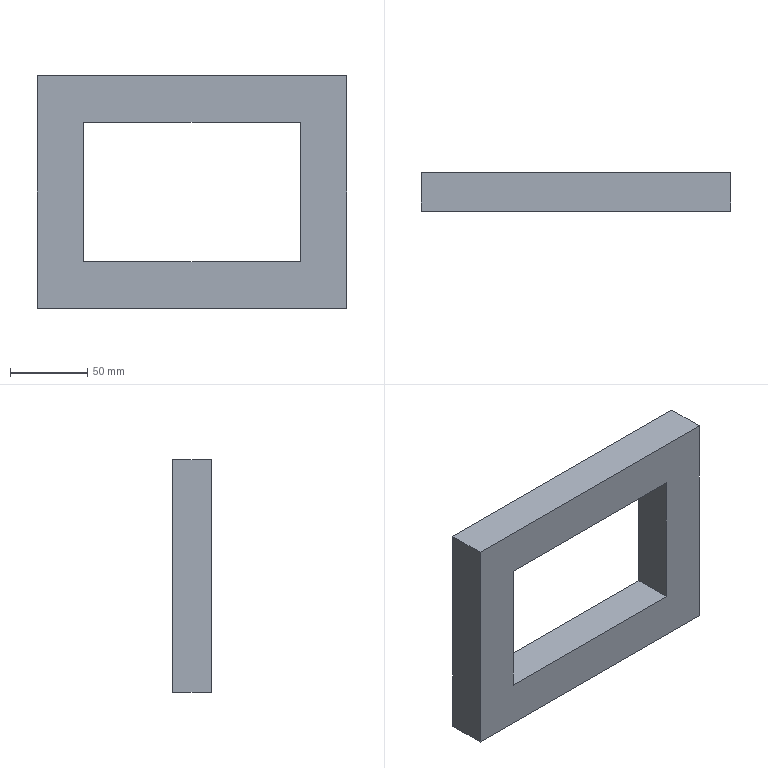Part | SolidWorks | features Extrusion 1, HoleWzd 1, ICE 1 | 1 solid | 46 faces | box 200 x 25 x 150 mm | volume 430967 mm3 | cone 24 | cylinder 12 | plane 10 | commonest cylinder face diameters 6.8 x12
STEP:
#1=CARTESIAN_POINT('',(-85.,24.375,56.6));
#2=VERTEX_POINT('',#1);
#3=CARTESIAN_POINT('',(-85.,24.375,63.4));
#4=VERTEX_POINT('',#3);
#5=CARTESIAN_POINT('',(-85.,24.375,60.));
#6=DIRECTION('',(0.,1.,0.));
#7=DIRECTION('',(0.,0.,1.));
#8=AXIS2_PLACEMENT_3D('',#5,#6,#7);
#9=CIRCLE('',#8,3.4);
#10=EDGE_CURVE('',#2,#4,#9,.T.);
#11=ORIENTED_EDGE('',*,*,#10,.F.);
#12=CARTESIAN_POINT('',(-85.,25.,55.975));
#13=VERTEX_POINT('',#12);
#14=CARTESIAN_POINT('',(-85.,25.,55.975));
#15=DIRECTION('',(0.,0.7071,-0.7071));
#16=VECTOR('',#15,1000.);
#17=LINE('',#14,#16);
#18=EDGE_CURVE('',#2,#13,#17,.T.);
#19=ORIENTED_EDGE('',*,*,#18,.T.);
#20=CARTESIAN_POINT('',(-85.,25.,64.025));
#21=VERTEX_POINT('',#20);
#22=CARTESIAN_POINT('',(-85.,25.,60.));
#23=DIRECTION('',(0.,1.,0.));
#24=DIRECTION('',(0.,0.,1.));
#25=AXIS2_PLACEMENT_3D('',#22,#23,#24);
#26=CIRCLE('',#25,4.025);
#27=EDGE_CURVE('',#13,#21,#26,.T.);
#28=ORIENTED_EDGE('',*,*,#27,.T.);
#29=CARTESIAN_POINT('',(-85.,25.,64.025));
#30=DIRECTION('',(0.,0.7071,0.7071));
#31=VECTOR('',#30,1000.);
#32=LINE('',#29,#31);
#33=EDGE_CURVE('',#4,#21,#32,.T.);
#34=ORIENTED_EDGE('',*,*,#33,.F.);
#35=EDGE_LOOP('',(#11,#19,#28,#34));
#36=FACE_OUTER_BOUND('',#35,.T.);
#37=CARTESIAN_POINT('',(-85.,25.,60.));
#38=DIRECTION('',(0.,1.,0.));
#39=DIRECTION('',(0.,0.,1.));
#40=AXIS2_PLACEMENT_3D('',#37,#38,#39);
#41=CONICAL_SURFACE('',#40,4.025,0.7854);
#42=ADVANCED_FACE('',(#36),#41,.F.);
#43=CARTESIAN_POINT('',(-85.,7.293,56.6));
#44=VERTEX_POINT('',#43);
#45=CARTESIAN_POINT('',(-85.,7.293,63.4));
#46=VERTEX_POINT('',#45);
#47=CARTESIAN_POINT('',(-85.,7.293,60.));
#48=DIRECTION('',(0.,1.,0.));
#49=DIRECTION('',(0.,0.,1.));
#50=AXIS2_PLACEMENT_3D('',#47,#48,#49);
#51=CIRCLE('',#50,3.4);
#52=EDGE_CURVE('',#44,#46,#51,.T.);
#53=ORIENTED_EDGE('',*,*,#52,.F.);
#54=CARTESIAN_POINT('',(-85.,25.,56.6));
#55=DIRECTION('',(0.,1.,0.));
#56=VECTOR('',#55,1000.);
#57=LINE('',#54,#56);
#58=EDGE_CURVE('',#44,#2,#57,.T.);
#59=ORIENTED_EDGE('',*,*,#58,.T.);
#60=ORIENTED_EDGE('',*,*,#10,.T.);
#61=CARTESIAN_POINT('',(-85.,25.,63.4));
#62=DIRECTION('',(0.,1.,0.));
#63=VECTOR('',#62,1000.);
#64=LINE('',#61,#63);
#65=EDGE_CURVE('',#46,#4,#64,.T.);
#66=ORIENTED_EDGE('',*,*,#65,.F.);
#67=EDGE_LOOP('',(#53,#59,#60,#66));
#68=FACE_OUTER_BOUND('',#67,.T.);
#69=CARTESIAN_POINT('',(-85.,25.,60.));
#70=DIRECTION('',(0.,1.,0.));
#71=DIRECTION('',(0.,0.,1.));
#72=AXIS2_PLACEMENT_3D('',#69,#70,#71);
#73=CYLINDRICAL_SURFACE('',#72,3.4);
#74=ADVANCED_FACE('',(#68),#73,.F.);
#75=CARTESIAN_POINT('',(-85.,5.25,60.));
#76=VERTEX_POINT('',#75);
#77=CARTESIAN_POINT('',(-85.,7.293,63.4));
#78=DIRECTION('',(0.,0.515,0.8572));
#79=VECTOR('',#78,1000.);
#80=LINE('',#77,#79);
#81=EDGE_CURVE('',#76,#46,#80,.T.);
#82=ORIENTED_EDGE('',*,*,#81,.F.);
#83=CARTESIAN_POINT('',(-85.,7.293,56.6));
#84=DIRECTION('',(0.,0.515,-0.8572));
#85=VECTOR('',#84,1000.);
#86=LINE('',#83,#85);
#87=EDGE_CURVE('',#76,#44,#86,.T.);
#88=ORIENTED_EDGE('',*,*,#87,.T.);
#89=ORIENTED_EDGE('',*,*,#52,.T.);
#90=EDGE_LOOP('',(#82,#88,#89));
#91=FACE_OUTER_BOUND('',#90,.T.);
#92=CARTESIAN_POINT('',(-85.,7.293,60.));
#93=DIRECTION('',(0.,1.,0.));
#94=DIRECTION('',(0.,0.,1.));
#95=AXIS2_PLACEMENT_3D('',#92,#93,#94);
#96=CONICAL_SURFACE('',#95,3.4,1.03);
#97=ADVANCED_FACE('',(#91),#96,.F.);
#98=CARTESIAN_POINT('',(0.,24.375,56.6));
#99=VERTEX_POINT('',#98);
#100=CARTESIAN_POINT('',(0.,24.375,63.4));
#101=VERTEX_POINT('',#100);
#102=CARTESIAN_POINT('',(0.,24.375,60.));
#103=DIRECTION('',(0.,1.,0.));
#104=DIRECTION('',(0.,0.,1.));
#105=AXIS2_PLACEMENT_3D('',#102,#103,#104);
#106=CIRCLE('',#105,3.4);
#107=EDGE_CURVE('',#99,#101,#106,.T.);
#108=ORIENTED_EDGE('',*,*,#107,.F.);
#109=CARTESIAN_POINT('',(0.,25.,55.975));
#110=VERTEX_POINT('',#109);
#111=CARTESIAN_POINT('',(0.,25.,55.975));
#112=DIRECTION('',(0.,0.7071,-0.7071));
#113=VECTOR('',#112,1000.);
#114=LINE('',#111,#113);
#115=EDGE_CURVE('',#99,#110,#114,.T.);
#116=ORIENTED_EDGE('',*,*,#115,.T.);
#117=CARTESIAN_POINT('',(0.,25.,64.025));
#118=VERTEX_POINT('',#117);
#119=CARTESIAN_POINT('',(0.,25.,60.));
#120=DIRECTION('',(0.,1.,0.));
#121=DIRECTION('',(0.,0.,1.));
#122=AXIS2_PLACEMENT_3D('',#119,#120,#121);
#123=CIRCLE('',#122,4.025);
#124=EDGE_CURVE('',#110,#118,#123,.T.);
#125=ORIENTED_EDGE('',*,*,#124,.T.);
#126=CARTESIAN_POINT('',(0.,25.,64.025));
#127=DIRECTION('',(0.,0.7071,0.7071));
#128=VECTOR('',#127,1000.);
#129=LINE('',#126,#128);
#130=EDGE_CURVE('',#101,#118,#129,.T.);
#131=ORIENTED_EDGE('',*,*,#130,.F.);
#132=EDGE_LOOP('',(#108,#116,#125,#131));
#133=FACE_OUTER_BOUND('',#132,.T.);
#134=CARTESIAN_POINT('',(0.,25.,60.));
#135=DIRECTION('',(0.,1.,0.));
#136=DIRECTION('',(0.,0.,1.));
#137=AXIS2_PLACEMENT_3D('',#134,#135,#136);
#138=CONICAL_SURFACE('',#137,4.025,0.7854);
#139=ADVANCED_FACE('',(#133),#138,.F.);
#140=CARTESIAN_POINT('',(0.,7.293,56.6));
#141=VERTEX_POINT('',#140);
#142=CARTESIAN_POINT('',(0.,7.293,63.4));
#143=VERTEX_POINT('',#142);
#144=CARTESIAN_POINT('',(0.,7.293,60.));
#145=DIRECTION('',(0.,1.,0.));
#146=DIRECTION('',(0.,0.,1.));
#147=AXIS2_PLACEMENT_3D('',#144,#145,#146);
#148=CIRCLE('',#147,3.4);
#149=EDGE_CURVE('',#141,#143,#148,.T.);
#150=ORIENTED_EDGE('',*,*,#149,.F.);
#151=CARTESIAN_POINT('',(0.,25.,56.6));
#152=DIRECTION('',(0.,1.,0.));
#153=VECTOR('',#152,1000.);
#154=LINE('',#151,#153);
#155=EDGE_CURVE('',#141,#99,#154,.T.);
#156=ORIENTED_EDGE('',*,*,#155,.T.);
#157=ORIENTED_EDGE('',*,*,#107,.T.);
#158=CARTESIAN_POINT('',(0.,25.,63.4));
#159=DIRECTION('',(0.,1.,0.));
#160=VECTOR('',#159,1000.);
#161=LINE('',#158,#160);
#162=EDGE_CURVE('',#143,#101,#161,.T.);
#163=ORIENTED_EDGE('',*,*,#162,.F.);
#164=EDGE_LOOP('',(#150,#156,#157,#163));
#165=FACE_OUTER_BOUND('',#164,.T.);
#166=CARTESIAN_POINT('',(0.,25.,60.));
#167=DIRECTION('',(0.,1.,0.));
#168=DIRECTION('',(0.,0.,1.));
#169=AXIS2_PLACEMENT_3D('',#166,#167,#168);
#170=CYLINDRICAL_SURFACE('',#169,3.4);
#171=ADVANCED_FACE('',(#165),#170,.F.);
#172=CARTESIAN_POINT('',(0.,5.25,60.));
#173=VERTEX_POINT('',#172);
#174=CARTESIAN_POINT('',(0.,7.293,63.4));
#175=DIRECTION('',(0.,0.515,0.8572));
#176=VECTOR('',#175,1000.);
#177=LINE('',#174,#176);
#178=EDGE_CURVE('',#173,#143,#177,.T.);
#179=ORIENTED_EDGE('',*,*,#178,.F.);
#180=CARTESIAN_POINT('',(0.,7.293,56.6));
#181=DIRECTION('',(0.,0.515,-0.8572));
#182=VECTOR('',#181,1000.);
#183=LINE('',#180,#182);
#184=EDGE_CURVE('',#173,#141,#183,.T.);
#185=ORIENTED_EDGE('',*,*,#184,.T.);
#186=ORIENTED_EDGE('',*,*,#149,.T.);
#187=EDGE_LOOP('',(#179,#185,#186));
#188=FACE_OUTER_BOUND('',#187,.T.);
#189=CARTESIAN_POINT('',(0.,7.293,60.));
#190=DIRECTION('',(0.,1.,0.));
#191=DIRECTION('',(0.,0.,1.));
#192=AXIS2_PLACEMENT_3D('',#189,#190,#191);
#193=CONICAL_SURFACE('',#192,3.4,1.03);
#194=ADVANCED_FACE('',(#188),#193,.F.);
#195=CARTESIAN_POINT('',(85.,24.375,56.6));
#196=VERTEX_POINT('',#195);
#197=CARTESIAN_POINT('',(85.,24.375,63.4));
#198=VERTEX_POINT('',#197);
#199=CARTESIAN_POINT('',(85.,24.375,60.));
#200=DIRECTION('',(0.,1.,0.));
#201=DIRECTION('',(0.,0.,1.));
#202=AXIS2_PLACEMENT_3D('',#199,#200,#201);
#203=CIRCLE('',#202,3.4);
#204=EDGE_CURVE('',#196,#198,#203,.T.);
#205=ORIENTED_EDGE('',*,*,#204,.F.);
#206=CARTESIAN_POINT('',(85.,25.,55.975));
#207=VERTEX_POINT('',#206);
#208=CARTESIAN_POINT('',(85.,25.,55.975));
#209=DIRECTION('',(0.,0.7071,-0.7071));
#210=VECTOR('',#209,1000.);
#211=LINE('',#208,#210);
#212=EDGE_CURVE('',#196,#207,#211,.T.);
#213=ORIENTED_EDGE('',*,*,#212,.T.);
#214=CARTESIAN_POINT('',(85.,25.,64.025));
#215=VERTEX_POINT('',#214);
#216=CARTESIAN_POINT('',(85.,25.,60.));
#217=DIRECTION('',(0.,1.,0.));
#218=DIRECTION('',(0.,0.,1.));
#219=AXIS2_PLACEMENT_3D('',#216,#217,#218);
#220=CIRCLE('',#219,4.025);
#221=EDGE_CURVE('',#207,#215,#220,.T.);
#222=ORIENTED_EDGE('',*,*,#221,.T.);
#223=CARTESIAN_POINT('',(85.,25.,64.025));
#224=DIRECTION('',(0.,0.7071,0.7071));
#225=VECTOR('',#224,1000.);
#226=LINE('',#223,#225);
#227=EDGE_CURVE('',#198,#215,#226,.T.);
#228=ORIENTED_EDGE('',*,*,#227,.F.);
#229=EDGE_LOOP('',(#205,#213,#222,#228));
#230=FACE_OUTER_BOUND('',#229,.T.);
#231=CARTESIAN_POINT('',(85.,25.,60.));
#232=DIRECTION('',(0.,1.,0.));
#233=DIRECTION('',(0.,0.,1.));
#234=AXIS2_PLACEMENT_3D('',#231,#232,#233);
#235=CONICAL_SURFACE('',#234,4.025,0.7854);
#236=ADVANCED_FACE('',(#230),#235,.F.);
#237=CARTESIAN_POINT('',(85.,7.293,56.6));
#238=VERTEX_POINT('',#237);
#239=CARTESIAN_POINT('',(85.,7.293,63.4));
#240=VERTEX_POINT('',#239);
#241=CARTESIAN_POINT('',(85.,7.293,60.));
#242=DIRECTION('',(0.,1.,0.));
#243=DIRECTION('',(0.,0.,1.));
#244=AXIS2_PLACEMENT_3D('',#241,#242,#243);
#245=CIRCLE('',#244,3.4);
#246=EDGE_CURVE('',#238,#240,#245,.T.);
#247=ORIENTED_EDGE('',*,*,#246,.F.);
#248=CARTESIAN_POINT('',(85.,25.,56.6));
#249=DIRECTION('',(0.,1.,0.));
#250=VECTOR('',#249,1000.);
#251=LINE('',#248,#250);
#252=EDGE_CURVE('',#238,#196,#251,.T.);
#253=ORIENTED_EDGE('',*,*,#252,.T.);
#254=ORIENTED_EDGE('',*,*,#204,.T.);
#255=CARTESIAN_POINT('',(85.,25.,63.4));
#256=DIRECTION('',(0.,1.,0.));
#257=VECTOR('',#256,1000.);
#258=LINE('',#255,#257);
#259=EDGE_CURVE('',#240,#198,#258,.T.);
#260=ORIENTED_EDGE('',*,*,#259,.F.);
#261=EDGE_LOOP('',(#247,#253,#254,#260));
#262=FACE_OUTER_BOUND('',#261,.T.);
#263=CARTESIAN_POINT('',(85.,25.,60.));
#264=DIRECTION('',(0.,1.,0.));
#265=DIRECTION('',(0.,0.,1.));
#266=AXIS2_PLACEMENT_3D('',#263,#264,#265);
#267=CYLINDRICAL_SURFACE('',#266,3.4);
#268=ADVANCED_FACE('',(#262),#267,.F.);
#269=CARTESIAN_POINT('',(85.,5.25,60.));
#270=VERTEX_POINT('',#269);
#271=CARTESIAN_POINT('',(85.,7.293,63.4));
#272=DIRECTION('',(0.,0.515,0.8572));
#273=VECTOR('',#272,1000.);
#274=LINE('',#271,#273);
#275=EDGE_CURVE('',#270,#240,#274,.T.);
#276=ORIENTED_EDGE('',*,*,#275,.F.);
#277=CARTESIAN_POINT('',(85.,7.293,56.6));
#278=DIRECTION('',(0.,0.515,-0.8572));
#279=VECTOR('',#278,1000.);
#280=LINE('',#277,#279);
#281=EDGE_CURVE('',#270,#238,#280,.T.);
#282=ORIENTED_EDGE('',*,*,#281,.T.);
#283=ORIENTED_EDGE('',*,*,#246,.T.);
#284=EDGE_LOOP('',(#276,#282,#283));
#285=FACE_OUTER_BOUND('',#284,.T.);
#286=CARTESIAN_POINT('',(85.,7.293,60.));
#287=DIRECTION('',(0.,1.,0.));
#288=DIRECTION('',(0.,0.,1.));
#289=AXIS2_PLACEMENT_3D('',#286,#287,#288);
#290=CONICAL_SURFACE('',#289,3.4,1.03);
#291=ADVANCED_FACE('',(#285),#290,.F.);
#292=CARTESIAN_POINT('',(85.,24.375,-63.4));
#293=VERTEX_POINT('',#292);
#294=CARTESIAN_POINT('',(85.,24.375,-56.6));
#295=VERTEX_POINT('',#294);
#296=CARTESIAN_POINT('',(85.,24.375,-60.));
#297=DIRECTION('',(0.,1.,0.));
#298=DIRECTION('',(0.,0.,1.));
#299=AXIS2_PLACEMENT_3D('',#296,#297,#298);
#300=CIRCLE('',#299,3.4);
#301=EDGE_CURVE('',#293,#295,#300,.T.);
#302=ORIENTED_EDGE('',*,*,#301,.F.);
#303=CARTESIAN_POINT('',(85.,25.,-64.025));
#304=VERTEX_POINT('',#303);
#305=CARTESIAN_POINT('',(85.,25.,-64.025));
#306=DIRECTION('',(0.,0.7071,-0.7071));
#307=VECTOR('',#306,1000.);
#308=LINE('',#305,#307);
#309=EDGE_CURVE('',#293,#304,#308,.T.);
#310=ORIENTED_EDGE('',*,*,#309,.T.);
#311=CARTESIAN_POINT('',(85.,25.,-55.975));
#312=VERTEX_POINT('',#311);
#313=CARTESIAN_POINT('',(85.,25.,-60.));
#314=DIRECTION('',(0.,1.,0.));
#315=DIRECTION('',(0.,0.,1.));
#316=AXIS2_PLACEMENT_3D('',#313,#314,#315);
#317=CIRCLE('',#316,4.025);
#318=EDGE_CURVE('',#304,#312,#317,.T.);
#319=ORIENTED_EDGE('',*,*,#318,.T.);
#320=CARTESIAN_POINT('',(85.,25.,-55.975));
#321=DIRECTION('',(0.,0.7071,0.7071));
#322=VECTOR('',#321,1000.);
#323=LINE('',#320,#322);
#324=EDGE_CURVE('',#295,#312,#323,.T.);
#325=ORIENTED_EDGE('',*,*,#324,.F.);
#326=EDGE_LOOP('',(#302,#310,#319,#325));
#327=FACE_OUTER_BOUND('',#326,.T.);
#328=CARTESIAN_POINT('',(85.,25.,-60.));
#329=DIRECTION('',(0.,1.,0.));
#330=DIRECTION('',(0.,0.,1.));
#331=AXIS2_PLACEMENT_3D('',#328,#329,#330);
#332=CONICAL_SURFACE('',#331,4.025,0.7854);
#333=ADVANCED_FACE('',(#327),#332,.F.);
#334=CARTESIAN_POINT('',(85.,7.293,-63.4));
#335=VERTEX_POINT('',#334);
#336=CARTESIAN_POINT('',(85.,7.293,-56.6));
#337=VERTEX_POINT('',#336);
#338=CARTESIAN_POINT('',(85.,7.293,-60.));
#339=DIRECTION('',(0.,1.,0.));
#340=DIRECTION('',(0.,0.,1.));
#341=AXIS2_PLACEMENT_3D('',#338,#339,#340);
#342=CIRCLE('',#341,3.4);
#343=EDGE_CURVE('',#335,#337,#342,.T.);
#344=ORIENTED_EDGE('',*,*,#343,.F.);
#345=CARTESIAN_POINT('',(85.,25.,-63.4));
#346=DIRECTION('',(0.,1.,0.));
#347=VECTOR('',#346,1000.);
#348=LINE('',#345,#347);
#349=EDGE_CURVE('',#335,#293,#348,.T.);
#350=ORIENTED_EDGE('',*,*,#349,.T.);
#351=ORIENTED_EDGE('',*,*,#301,.T.);
#352=CARTESIAN_POINT('',(85.,25.,-56.6));
#353=DIRECTION('',(0.,1.,0.));
#354=VECTOR('',#353,1000.);
#355=LINE('',#352,#354);
#356=EDGE_CURVE('',#337,#295,#355,.T.);
#357=ORIENTED_EDGE('',*,*,#356,.F.);
#358=EDGE_LOOP('',(#344,#350,#351,#357));
#359=FACE_OUTER_BOUND('',#358,.T.);
#360=CARTESIAN_POINT('',(85.,25.,-60.));
#361=DIRECTION('',(0.,1.,0.));
#362=DIRECTION('',(0.,0.,1.));
#363=AXIS2_PLACEMENT_3D('',#360,#361,#362);
#364=CYLINDRICAL_SURFACE('',#363,3.4);
#365=ADVANCED_FACE('',(#359),#364,.F.);
#366=CARTESIAN_POINT('',(85.,5.25,-60.));
#367=VERTEX_POINT('',#366);
#368=CARTESIAN_POINT('',(85.,7.293,-56.6));
#369=DIRECTION('',(0.,0.515,0.8572));
#370=VECTOR('',#369,1000.);
#371=LINE('',#368,#370);
#372=EDGE_CURVE('',#367,#337,#371,.T.);
#373=ORIENTED_EDGE('',*,*,#372,.F.);
#374=CARTESIAN_POINT('',(85.,7.293,-63.4));
#375=DIRECTION('',(0.,0.515,-0.8572));
#376=VECTOR('',#375,1000.);
#377=LINE('',#374,#376);
#378=EDGE_CURVE('',#367,#335,#377,.T.);
#379=ORIENTED_EDGE('',*,*,#378,.T.);
#380=ORIENTED_EDGE('',*,*,#343,.T.);
#381=EDGE_LOOP('',(#373,#379,#380));
#382=FACE_OUTER_BOUND('',#381,.T.);
#383=CARTESIAN_POINT('',(85.,7.293,-60.));
#384=DIRECTION('',(0.,1.,0.));
#385=DIRECTION('',(0.,0.,1.));
#386=AXIS2_PLACEMENT_3D('',#383,#384,#385);
#387=CONICAL_SURFACE('',#386,3.4,1.03);
#388=ADVANCED_FACE('',(#382),#387,.F.);
#389=CARTESIAN_POINT('',(0.,24.375,-63.4));
#390=VERTEX_POINT('',#389);
#391=CARTESIAN_POINT('',(0.,24.375,-56.6));
#392=VERTEX_POINT('',#391);
#393=CARTESIAN_POINT('',(0.,24.375,-60.));
#394=DIRECTION('',(0.,1.,0.));
#395=DIRECTION('',(0.,0.,1.));
#396=AXIS2_PLACEMENT_3D('',#393,#394,#395);
#397=CIRCLE('',#396,3.4);
#398=EDGE_CURVE('',#390,#392,#397,.T.);
#399=ORIENTED_EDGE('',*,*,#398,.F.);
#400=CARTESIAN_POINT('',(0.,25.,-64.025));
#401=VERTEX_POINT('',#400);
#402=CARTESIAN_POINT('',(0.,25.,-64.025));
#403=DIRECTION('',(0.,0.7071,-0.7071));
#404=VECTOR('',#403,1000.);
#405=LINE('',#402,#404);
#406=EDGE_CURVE('',#390,#401,#405,.T.);
#407=ORIENTED_EDGE('',*,*,#406,.T.);
#408=CARTESIAN_POINT('',(0.,25.,-55.975));
#409=VERTEX_POINT('',#408);
#410=CARTESIAN_POINT('',(0.,25.,-60.));
#411=DIRECTION('',(0.,1.,0.));
#412=DIRECTION('',(0.,0.,1.));
#413=AXIS2_PLACEMENT_3D('',#410,#411,#412);
#414=CIRCLE('',#413,4.025);
#415=EDGE_CURVE('',#401,#409,#414,.T.);
#416=ORIENTED_EDGE('',*,*,#415,.T.);
#417=CARTESIAN_POINT('',(0.,25.,-55.975));
#418=DIRECTION('',(0.,0.7071,0.7071));
#419=VECTOR('',#418,1000.);
#420=LINE('',#417,#419);
#421=EDGE_CURVE('',#392,#409,#420,.T.);
#422=ORIENTED_EDGE('',*,*,#421,.F.);
#423=EDGE_LOOP('',(#399,#407,#416,#422));
#424=FACE_OUTER_BOUND('',#423,.T.);
#425=CARTESIAN_POINT('',(0.,25.,-60.));
#426=DIRECTION('',(0.,1.,0.));
#427=DIRECTION('',(0.,0.,1.));
#428=AXIS2_PLACEMENT_3D('',#425,#426,#427);
#429=CONICAL_SURFACE('',#428,4.025,0.7854);
#430=ADVANCED_FACE('',(#424),#429,.F.);
#431=CARTESIAN_POINT('',(0.,7.293,-63.4));
#432=VERTEX_POINT('',#431);
#433=CARTESIAN_POINT('',(0.,7.293,-56.6));
#434=VERTEX_POINT('',#433);
#435=CARTESIAN_POINT('',(0.,7.293,-60.));
#436=DIRECTION('',(0.,1.,0.));
#437=DIRECTION('',(0.,0.,1.));
#438=AXIS2_PLACEMENT_3D('',#435,#436,#437);
#439=CIRCLE('',#438,3.4);
#440=EDGE_CURVE('',#432,#434,#439,.T.);
#441=ORIENTED_EDGE('',*,*,#440,.F.);
#442=CARTESIAN_POINT('',(0.,25.,-63.4));
#443=DIRECTION('',(0.,1.,0.));
#444=VECTOR('',#443,1000.);
#445=LINE('',#442,#444);
#446=EDGE_CURVE('',#432,#390,#445,.T.);
#447=ORIENTED_EDGE('',*,*,#446,.T.);
#448=ORIENTED_EDGE('',*,*,#398,.T.);
#449=CARTESIAN_POINT('',(0.,25.,-56.6));
#450=DIRECTION('',(0.,1.,0.));
#451=VECTOR('',#450,1000.);
#452=LINE('',#449,#451);
#453=EDGE_CURVE('',#434,#392,#452,.T.);
#454=ORIENTED_EDGE('',*,*,#453,.F.);
#455=EDGE_LOOP('',(#441,#447,#448,#454));
#456=FACE_OUTER_BOUND('',#455,.T.);
#457=CARTESIAN_POINT('',(0.,25.,-60.));
#458=DIRECTION('',(0.,1.,0.));
#459=DIRECTION('',(0.,0.,1.));
#460=AXIS2_PLACEMENT_3D('',#457,#458,#459);
#461=CYLINDRICAL_SURFACE('',#460,3.4);
#462=ADVANCED_FACE('',(#456),#461,.F.);
#463=CARTESIAN_POINT('',(0.,5.25,-60.));
#464=VERTEX_POINT('',#463);
#465=CARTESIAN_POINT('',(0.,7.293,-56.6));
#466=DIRECTION('',(0.,0.515,0.8572));
#467=VECTOR('',#466,1000.);
#468=LINE('',#465,#467);
#469=EDGE_CURVE('',#464,#434,#468,.T.);
#470=ORIENTED_EDGE('',*,*,#469,.F.);
#471=CARTESIAN_POINT('',(0.,7.293,-63.4));
#472=DIRECTION('',(0.,0.515,-0.8572));
#473=VECTOR('',#472,1000.);
#474=LINE('',#471,#473);
#475=EDGE_CURVE('',#464,#432,#474,.T.);
#476=ORIENTED_EDGE('',*,*,#475,.T.);
#477=ORIENTED_EDGE('',*,*,#440,.T.);
#478=EDGE_LOOP('',(#470,#476,#477));
#479=FACE_OUTER_BOUND('',#478,.T.);
#480=CARTESIAN_POINT('',(0.,7.293,-60.));
#481=DIRECTION('',(0.,1.,0.));
#482=DIRECTION('',(0.,0.,1.));
#483=AXIS2_PLACEMENT_3D('',#480,#481,#482);
#484=CONICAL_SURFACE('',#483,3.4,1.03);
#485=ADVANCED_FACE('',(#479),#484,.F.);
#486=CARTESIAN_POINT('',(-85.,24.375,-63.4));
#487=VERTEX_POINT('',#486);
#488=CARTESIAN_POINT('',(-85.,24.375,-56.6));
#489=VERTEX_POINT('',#488);
#490=CARTESIAN_POINT('',(-85.,24.375,-60.));
#491=DIRECTION('',(0.,1.,0.));
#492=DIRECTION('',(0.,0.,1.));
#493=AXIS2_PLACEMENT_3D('',#490,#491,#492);
#494=CIRCLE('',#493,3.4);
#495=EDGE_CURVE('',#487,#489,#494,.T.);
#496=ORIENTED_EDGE('',*,*,#495,.F.);
#497=CARTESIAN_POINT('',(-85.,25.,-64.025));
#498=VERTEX_POINT('',#497);
#499=CARTESIAN_POINT('',(-85.,25.,-64.025));
#500=DIRECTION('',(0.,0.7071,-0.7071));
#501=VECTOR('',#500,1000.);
#502=LINE('',#499,#501);
#503=EDGE_CURVE('',#487,#498,#502,.T.);
#504=ORIENTED_EDGE('',*,*,#503,.T.);
#505=CARTESIAN_POINT('',(-85.,25.,-55.975));
#506=VERTEX_POINT('',#505);
#507=CARTESIAN_POINT('',(-85.,25.,-60.));
#508=DIRECTION('',(0.,1.,0.));
#509=DIRECTION('',(0.,0.,1.));
#510=AXIS2_PLACEMENT_3D('',#507,#508,#509);
#511=CIRCLE('',#510,4.025);
#512=EDGE_CURVE('',#498,#506,#511,.T.);
#513=ORIENTED_EDGE('',*,*,#512,.T.);
#514=CARTESIAN_POINT('',(-85.,25.,-55.975));
#515=DIRECTION('',(0.,0.7071,0.7071));
#516=VECTOR('',#515,1000.);
#517=LINE('',#514,#516);
#518=EDGE_CURVE('',#489,#506,#517,.T.);
#519=ORIENTED_EDGE('',*,*,#518,.F.);
#520=EDGE_LOOP('',(#496,#504,#513,#519));
#521=FACE_OUTER_BOUND('',#520,.T.);
#522=CARTESIAN_POINT('',(-85.,25.,-60.));
#523=DIRECTION('',(0.,1.,0.));
#524=DIRECTION('',(0.,0.,1.));
#525=AXIS2_PLACEMENT_3D('',#522,#523,#524);
#526=CONICAL_SURFACE('',#525,4.025,0.7854);
#527=ADVANCED_FACE('',(#521),#526,.F.);
#528=CARTESIAN_POINT('',(-85.,7.293,-63.4));
#529=VERTEX_POINT('',#528);
#530=CARTESIAN_POINT('',(-85.,7.293,-56.6));
#531=VERTEX_POINT('',#530);
#532=CARTESIAN_POINT('',(-85.,7.293,-60.));
#533=DIRECTION('',(0.,1.,0.));
#534=DIRECTION('',(0.,0.,1.));
#535=AXIS2_PLACEMENT_3D('',#532,#533,#534);
#536=CIRCLE('',#535,3.4);
#537=EDGE_CURVE('',#529,#531,#536,.T.);
#538=ORIENTED_EDGE('',*,*,#537,.F.);
#539=CARTESIAN_POINT('',(-85.,25.,-63.4));
#540=DIRECTION('',(0.,1.,0.));
#541=VECTOR('',#540,1000.);
#542=LINE('',#539,#541);
#543=EDGE_CURVE('',#529,#487,#542,.T.);
#544=ORIENTED_EDGE('',*,*,#543,.T.);
#545=ORIENTED_EDGE('',*,*,#495,.T.);
#546=CARTESIAN_POINT('',(-85.,25.,-56.6));
#547=DIRECTION('',(0.,1.,0.));
#548=VECTOR('',#547,1000.);
#549=LINE('',#546,#548);
#550=EDGE_CURVE('',#531,#489,#549,.T.);
#551=ORIENTED_EDGE('',*,*,#550,.F.);
#552=EDGE_LOOP('',(#538,#544,#545,#551));
#553=FACE_OUTER_BOUND('',#552,.T.);
#554=CARTESIAN_POINT('',(-85.,25.,-60.));
#555=DIRECTION('',(0.,1.,0.));
#556=DIRECTION('',(0.,0.,1.));
#557=AXIS2_PLACEMENT_3D('',#554,#555,#556);
#558=CYLINDRICAL_SURFACE('',#557,3.4);
#559=ADVANCED_FACE('',(#553),#558,.F.);
#560=CARTESIAN_POINT('',(-85.,5.25,-60.));
#561=VERTEX_POINT('',#560);
#562=CARTESIAN_POINT('',(-85.,7.293,-56.6));
#563=DIRECTION('',(0.,0.515,0.8572));
#564=VECTOR('',#563,1000.);
#565=LINE('',#562,#564);
#566=EDGE_CURVE('',#561,#531,#565,.T.);
#567=ORIENTED_EDGE('',*,*,#566,.F.);
#568=CARTESIAN_POINT('',(-85.,7.293,-63.4));
#569=DIRECTION('',(0.,0.515,-0.8572));
#570=VECTOR('',#569,1000.);
#571=LINE('',#568,#570);
#572=EDGE_CURVE('',#561,#529,#571,.T.);
#573=ORIENTED_EDGE('',*,*,#572,.T.);
#574=ORIENTED_EDGE('',*,*,#537,.T.);
#575=EDGE_LOOP('',(#567,#573,#574));
#576=FACE_OUTER_BOUND('',#575,.T.);
#577=CARTESIAN_POINT('',(-85.,7.293,-60.));
#578=DIRECTION('',(0.,1.,0.));
#579=DIRECTION('',(0.,0.,1.));
#580=AXIS2_PLACEMENT_3D('',#577,#578,#579);
#581=CONICAL_SURFACE('',#580,3.4,1.03);
#582=ADVANCED_FACE('',(#576),#581,.F.);
#583=CARTESIAN_POINT('',(100.,0.,75.));
#584=VERTEX_POINT('',#583);
#585=CARTESIAN_POINT('',(100.,0.,-75.));
#586=VERTEX_POINT('',#585);
#587=CARTESIAN_POINT('',(100.,0.,-75.));
#588=DIRECTION('',(0.,0.,-1.));
#589=VECTOR('',#588,1000.);
#590=LINE('',#587,#589);
#591=EDGE_CURVE('',#584,#586,#590,.T.);
#592=ORIENTED_EDGE('',*,*,#591,.T.);
#593=CARTESIAN_POINT('',(100.,25.,-75.));
#594=VERTEX_POINT('',#593);
#595=CARTESIAN_POINT('',(100.,25.,-75.));
#596=DIRECTION('',(0.,-1.,0.));
#597=VECTOR('',#596,1000.);
#598=LINE('',#595,#597);
#599=EDGE_CURVE('',#594,#586,#598,.T.);
#600=ORIENTED_EDGE('',*,*,#599,.F.);
#601=CARTESIAN_POINT('',(100.,25.,75.));
#602=VERTEX_POINT('',#601);
#603=CARTESIAN_POINT('',(100.,25.,-75.));
#604=DIRECTION('',(0.,0.,-1.));
#605=VECTOR('',#604,1000.);
#606=LINE('',#603,#605);
#607=EDGE_CURVE('',#602,#594,#606,.T.);
#608=ORIENTED_EDGE('',*,*,#607,.F.);
#609=CARTESIAN_POINT('',(100.,25.,75.));
#610=DIRECTION('',(0.,-1.,0.));
#611=VECTOR('',#610,1000.);
#612=LINE('',#609,#611);
#613=EDGE_CURVE('',#602,#584,#612,.T.);
#614=ORIENTED_EDGE('',*,*,#613,.T.);
#615=EDGE_LOOP('',(#592,#600,#608,#614));
#616=FACE_OUTER_BOUND('',#615,.T.);
#617=CARTESIAN_POINT('',(100.,25.,-75.));
#618=DIRECTION('',(-1.,0.,0.));
#619=DIRECTION('',(0.,0.,1.));
#620=AXIS2_PLACEMENT_3D('',#617,#618,#619);
#621=PLANE('',#620);
#622=ADVANCED_FACE('',(#616),#621,.F.);
#623=CARTESIAN_POINT('',(-100.,0.,-75.));
#624=VERTEX_POINT('',#623);
#625=CARTESIAN_POINT('',(-100.,0.,-75.));
#626=DIRECTION('',(-1.,0.,0.));
#627=VECTOR('',#626,1000.);
#628=LINE('',#625,#627);
#629=EDGE_CURVE('',#586,#624,#628,.T.);
#630=ORIENTED_EDGE('',*,*,#629,.T.);
#631=CARTESIAN_POINT('',(-100.,25.,-75.));
#632=VERTEX_POINT('',#631);
#633=CARTESIAN_POINT('',(-100.,25.,-75.));
#634=DIRECTION('',(0.,-1.,0.));
#635=VECTOR('',#634,1000.);
#636=LINE('',#633,#635);
#637=EDGE_CURVE('',#632,#624,#636,.T.);
#638=ORIENTED_EDGE('',*,*,#637,.F.);
#639=CARTESIAN_POINT('',(-100.,25.,-75.));
#640=DIRECTION('',(-1.,0.,0.));
#641=VECTOR('',#640,1000.);
#642=LINE('',#639,#641);
#643=EDGE_CURVE('',#594,#632,#642,.T.);
#644=ORIENTED_EDGE('',*,*,#643,.F.);
#645=ORIENTED_EDGE('',*,*,#599,.T.);
#646=EDGE_LOOP('',(#630,#638,#644,#645));
#647=FACE_OUTER_BOUND('',#646,.T.);
#648=CARTESIAN_POINT('',(-100.,25.,-75.));
#649=DIRECTION('',(0.,0.,1.));
#650=DIRECTION('',(1.,0.,0.));
#651=AXIS2_PLACEMENT_3D('',#648,#649,#650);
#652=PLANE('',#651);
#653=ADVANCED_FACE('',(#647),#652,.F.);
#654=CARTESIAN_POINT('',(-100.,0.,75.));
#655=VERTEX_POINT('',#654);
#656=CARTESIAN_POINT('',(-100.,0.,-75.));
#657=DIRECTION('',(0.,0.,1.));
#658=VECTOR('',#657,1000.);
#659=LINE('',#656,#658);
#660=EDGE_CURVE('',#624,#655,#659,.T.);
#661=ORIENTED_EDGE('',*,*,#660,.T.);
#662=CARTESIAN_POINT('',(-100.,25.,75.));
#663=VERTEX_POINT('',#662);
#664=CARTESIAN_POINT('',(-100.,25.,75.));
#665=DIRECTION('',(0.,-1.,0.));
#666=VECTOR('',#665,1000.);
#667=LINE('',#664,#666);
#668=EDGE_CURVE('',#663,#655,#667,.T.);
#669=ORIENTED_EDGE('',*,*,#668,.F.);
#670=CARTESIAN_POINT('',(-100.,25.,-75.));
#671=DIRECTION('',(0.,0.,1.));
#672=VECTOR('',#671,1000.);
#673=LINE('',#670,#672);
#674=EDGE_CURVE('',#632,#663,#673,.T.);
#675=ORIENTED_EDGE('',*,*,#674,.F.);
#676=ORIENTED_EDGE('',*,*,#637,.T.);
#677=EDGE_LOOP('',(#661,#669,#675,#676));
#678=FACE_OUTER_BOUND('',#677,.T.);
#679=CARTESIAN_POINT('',(-100.,25.,-75.));
#680=DIRECTION('',(1.,0.,0.));
#681=DIRECTION('',(0.,0.,-1.));
#682=AXIS2_PLACEMENT_3D('',#679,#680,#681);
#683=PLANE('',#682);
#684=ADVANCED_FACE('',(#678),#683,.F.);
#685=CARTESIAN_POINT('',(-100.,0.,75.));
#686=DIRECTION('',(1.,0.,0.));
#687=VECTOR('',#686,1000.);
#688=LINE('',#685,#687);
#689=EDGE_CURVE('',#655,#584,#688,.T.);
#690=ORIENTED_EDGE('',*,*,#689,.T.);
#691=ORIENTED_EDGE('',*,*,#613,.F.);
#692=CARTESIAN_POINT('',(-100.,25.,75.));
#693=DIRECTION('',(1.,0.,0.));
#694=VECTOR('',#693,1000.);
#695=LINE('',#692,#694);
#696=EDGE_CURVE('',#663,#602,#695,.T.);
#697=ORIENTED_EDGE('',*,*,#696,.F.);
#698=ORIENTED_EDGE('',*,*,#668,.T.);
#699=EDGE_LOOP('',(#690,#691,#697,#698));
#700=FACE_OUTER_BOUND('',#699,.T.);
#701=CARTESIAN_POINT('',(-100.,25.,75.));
#702=DIRECTION('',(0.,0.,-1.));
#703=DIRECTION('',(-1.,0.,0.));
#704=AXIS2_PLACEMENT_3D('',#701,#702,#703);
#705=PLANE('',#704);
#706=ADVANCED_FACE('',(#700),#705,.F.);
#707=CARTESIAN_POINT('',(-70.,25.,-45.));
#708=VERTEX_POINT('',#707);
#709=CARTESIAN_POINT('',(-70.,25.,45.));
#710=VERTEX_POINT('',#709);
#711=CARTESIAN_POINT('',(-70.,25.,0.));
#712=DIRECTION('',(0.,0.,1.));
#713=VECTOR('',#712,1000.);
#714=LINE('',#711,#713);
#715=EDGE_CURVE('',#708,#710,#714,.T.);
#716=ORIENTED_EDGE('',*,*,#715,.F.);
#717=CARTESIAN_POINT('',(70.,25.,-45.));
#718=VERTEX_POINT('',#717);
#719=CARTESIAN_POINT('',(0.,25.,-45.));
#720=DIRECTION('',(-1.,0.,0.));
#721=VECTOR('',#720,1000.);
#722=LINE('',#719,#721);
#723=EDGE_CURVE('',#718,#708,#722,.T.);
#724=ORIENTED_EDGE('',*,*,#723,.F.);
#725=CARTESIAN_POINT('',(70.,25.,45.));
#726=VERTEX_POINT('',#725);
#727=CARTESIAN_POINT('',(70.,25.,0.));
#728=DIRECTION('',(0.,0.,-1.));
#729=VECTOR('',#728,1000.);
#730=LINE('',#727,#729);
#731=EDGE_CURVE('',#726,#718,#730,.T.);
#732=ORIENTED_EDGE('',*,*,#731,.F.);
#733=CARTESIAN_POINT('',(0.,25.,45.));
#734=DIRECTION('',(1.,0.,0.));
#735=VECTOR('',#734,1000.);
#736=LINE('',#733,#735);
#737=EDGE_CURVE('',#710,#726,#736,.T.);
#738=ORIENTED_EDGE('',*,*,#737,.F.);
#739=EDGE_LOOP('',(#716,#724,#732,#738));
#740=FACE_BOUND('',#739,.T.);
#741=CARTESIAN_POINT('',(-85.,25.,60.));
#742=DIRECTION('',(0.,1.,0.));
#743=DIRECTION('',(0.,0.,1.));
#744=AXIS2_PLACEMENT_3D('',#741,#742,#743);
#745=CIRCLE('',#744,4.025);
#746=EDGE_CURVE('',#21,#13,#745,.T.);
#747=ORIENTED_EDGE('',*,*,#746,.F.);
#748=ORIENTED_EDGE('',*,*,#27,.F.);
#749=EDGE_LOOP('',(#747,#748));
#750=FACE_BOUND('',#749,.T.);
#751=CARTESIAN_POINT('',(0.,25.,60.));
#752=DIRECTION('',(0.,1.,0.));
#753=DIRECTION('',(0.,0.,1.));
#754=AXIS2_PLACEMENT_3D('',#751,#752,#753);
#755=CIRCLE('',#754,4.025);
#756=EDGE_CURVE('',#118,#110,#755,.T.);
#757=ORIENTED_EDGE('',*,*,#756,.F.);
#758=ORIENTED_EDGE('',*,*,#124,.F.);
#759=EDGE_LOOP('',(#757,#758));
#760=FACE_BOUND('',#759,.T.);
#761=CARTESIAN_POINT('',(85.,25.,60.));
#762=DIRECTION('',(0.,1.,0.));
#763=DIRECTION('',(0.,0.,1.));
#764=AXIS2_PLACEMENT_3D('',#761,#762,#763);
#765=CIRCLE('',#764,4.025);
#766=EDGE_CURVE('',#215,#207,#765,.T.);
#767=ORIENTED_EDGE('',*,*,#766,.F.);
#768=ORIENTED_EDGE('',*,*,#221,.F.);
#769=EDGE_LOOP('',(#767,#768));
#770=FACE_BOUND('',#769,.T.);
#771=CARTESIAN_POINT('',(85.,25.,-60.));
#772=DIRECTION('',(0.,1.,0.));
#773=DIRECTION('',(0.,0.,1.));
#774=AXIS2_PLACEMENT_3D('',#771,#772,#773);
#775=CIRCLE('',#774,4.025);
#776=EDGE_CURVE('',#312,#304,#775,.T.);
#777=ORIENTED_EDGE('',*,*,#776,.F.);
#778=ORIENTED_EDGE('',*,*,#318,.F.);
#779=EDGE_LOOP('',(#777,#778));
#780=FACE_BOUND('',#779,.T.);
#781=CARTESIAN_POINT('',(0.,25.,-60.));
#782=DIRECTION('',(0.,1.,0.));
#783=DIRECTION('',(0.,0.,1.));
#784=AXIS2_PLACEMENT_3D('',#781,#782,#783);
#785=CIRCLE('',#784,4.025);
#786=EDGE_CURVE('',#409,#401,#785,.T.);
#787=ORIENTED_EDGE('',*,*,#786,.F.);
#788=ORIENTED_EDGE('',*,*,#415,.F.);
#789=EDGE_LOOP('',(#787,#788));
#790=FACE_BOUND('',#789,.T.);
#791=CARTESIAN_POINT('',(-85.,25.,-60.));
#792=DIRECTION('',(0.,1.,0.));
#793=DIRECTION('',(0.,0.,1.));
#794=AXIS2_PLACEMENT_3D('',#791,#792,#793);
#795=CIRCLE('',#794,4.025);
#796=EDGE_CURVE('',#506,#498,#795,.T.);
#797=ORIENTED_EDGE('',*,*,#796,.F.);
#798=ORIENTED_EDGE('',*,*,#512,.F.);
#799=EDGE_LOOP('',(#797,#798));
#800=FACE_BOUND('',#799,.T.);
#801=ORIENTED_EDGE('',*,*,#607,.T.);
#802=ORIENTED_EDGE('',*,*,#643,.T.);
#803=ORIENTED_EDGE('',*,*,#674,.T.);
#804=ORIENTED_EDGE('',*,*,#696,.T.);
#805=EDGE_LOOP('',(#801,#802,#803,#804));
#806=FACE_OUTER_BOUND('',#805,.T.);
#807=CARTESIAN_POINT('',(0.,25.,0.));
#808=DIRECTION('',(0.,1.,0.));
#809=DIRECTION('',(0.,0.,1.));
#810=AXIS2_PLACEMENT_3D('',#807,#808,#809);
#811=PLANE('',#810);
#812=ADVANCED_FACE('',(#740,#750,#760,#770,#780,#790,#800,#806),#811,.T.);
#813=CARTESIAN_POINT('',(70.,0.,-45.));
#814=VERTEX_POINT('',#813);
#815=CARTESIAN_POINT('',(-70.,0.,-45.));
#816=VERTEX_POINT('',#815);
#817=CARTESIAN_POINT('',(70.,0.,-45.));
#818=DIRECTION('',(-1.,0.,0.));
#819=VECTOR('',#818,1000.);
#820=LINE('',#817,#819);
#821=EDGE_CURVE('',#814,#816,#820,.T.);
#822=ORIENTED_EDGE('',*,*,#821,.T.);
#823=CARTESIAN_POINT('',(-70.,0.,45.));
#824=VERTEX_POINT('',#823);
#825=CARTESIAN_POINT('',(-70.,0.,-45.));
#826=DIRECTION('',(0.,0.,1.));
#827=VECTOR('',#826,1000.);
#828=LINE('',#825,#827);
#829=EDGE_CURVE('',#816,#824,#828,.T.);
#830=ORIENTED_EDGE('',*,*,#829,.T.);
#831=CARTESIAN_POINT('',(70.,0.,45.));
#832=VERTEX_POINT('',#831);
#833=CARTESIAN_POINT('',(70.,0.,45.));
#834=DIRECTION('',(1.,0.,0.));
#835=VECTOR('',#834,1000.);
#836=LINE('',#833,#835);
#837=EDGE_CURVE('',#824,#832,#836,.T.);
#838=ORIENTED_EDGE('',*,*,#837,.T.);
#839=CARTESIAN_POINT('',(70.,0.,-45.));
#840=DIRECTION('',(0.,0.,-1.));
#841=VECTOR('',#840,1000.);
#842=LINE('',#839,#841);
#843=EDGE_CURVE('',#832,#814,#842,.T.);
#844=ORIENTED_EDGE('',*,*,#843,.T.);
#845=EDGE_LOOP('',(#822,#830,#838,#844));
#846=FACE_BOUND('',#845,.T.);
#847=ORIENTED_EDGE('',*,*,#591,.F.);
#848=ORIENTED_EDGE('',*,*,#689,.F.);
#849=ORIENTED_EDGE('',*,*,#660,.F.);
#850=ORIENTED_EDGE('',*,*,#629,.F.);
#851=EDGE_LOOP('',(#847,#848,#849,#850));
#852=FACE_OUTER_BOUND('',#851,.T.);
#853=CARTESIAN_POINT('',(0.,0.,0.));
#854=DIRECTION('',(0.,1.,0.));
#855=DIRECTION('',(0.,0.,1.));
#856=AXIS2_PLACEMENT_3D('',#853,#854,#855);
#857=PLANE('',#856);
#858=ADVANCED_FACE('',(#846,#852),#857,.F.);
#859=ORIENTED_EDGE('',*,*,#572,.F.);
#860=ORIENTED_EDGE('',*,*,#566,.T.);
#861=CARTESIAN_POINT('',(-85.,7.293,-60.));
#862=DIRECTION('',(0.,1.,0.));
#863=DIRECTION('',(0.,0.,1.));
#864=AXIS2_PLACEMENT_3D('',#861,#862,#863);
#865=CIRCLE('',#864,3.4);
#866=EDGE_CURVE('',#531,#529,#865,.T.);
#867=ORIENTED_EDGE('',*,*,#866,.T.);
#868=EDGE_LOOP('',(#859,#860,#867));
#869=FACE_OUTER_BOUND('',#868,.T.);
#870=CARTESIAN_POINT('',(-85.,7.293,-60.));
#871=DIRECTION('',(0.,1.,0.));
#872=DIRECTION('',(0.,0.,1.));
#873=AXIS2_PLACEMENT_3D('',#870,#871,#872);
#874=CONICAL_SURFACE('',#873,3.4,1.03);
#875=ADVANCED_FACE('',(#869),#874,.F.);
#876=ORIENTED_EDGE('',*,*,#543,.F.);
#877=ORIENTED_EDGE('',*,*,#866,.F.);
#878=ORIENTED_EDGE('',*,*,#550,.T.);
#879=CARTESIAN_POINT('',(-85.,24.375,-60.));
#880=DIRECTION('',(0.,1.,0.));
#881=DIRECTION('',(0.,0.,1.));
#882=AXIS2_PLACEMENT_3D('',#879,#880,#881);
#883=CIRCLE('',#882,3.4);
#884=EDGE_CURVE('',#489,#487,#883,.T.);
#885=ORIENTED_EDGE('',*,*,#884,.T.);
#886=EDGE_LOOP('',(#876,#877,#878,#885));
#887=FACE_OUTER_BOUND('',#886,.T.);
#888=CARTESIAN_POINT('',(-85.,25.,-60.));
#889=DIRECTION('',(0.,1.,0.));
#890=DIRECTION('',(0.,0.,1.));
#891=AXIS2_PLACEMENT_3D('',#888,#889,#890);
#892=CYLINDRICAL_SURFACE('',#891,3.4);
#893=ADVANCED_FACE('',(#887),#892,.F.);
#894=ORIENTED_EDGE('',*,*,#503,.F.);
#895=ORIENTED_EDGE('',*,*,#884,.F.);
#896=ORIENTED_EDGE('',*,*,#518,.T.);
#897=ORIENTED_EDGE('',*,*,#796,.T.);
#898=EDGE_LOOP('',(#894,#895,#896,#897));
#899=FACE_OUTER_BOUND('',#898,.T.);
#900=CARTESIAN_POINT('',(-85.,25.,-60.));
#901=DIRECTION('',(0.,1.,0.));
#902=DIRECTION('',(0.,0.,1.));
#903=AXIS2_PLACEMENT_3D('',#900,#901,#902);
#904=CONICAL_SURFACE('',#903,4.025,0.7854);
#905=ADVANCED_FACE('',(#899),#904,.F.);
#906=ORIENTED_EDGE('',*,*,#475,.F.);
#907=ORIENTED_EDGE('',*,*,#469,.T.);
#908=CARTESIAN_POINT('',(0.,7.293,-60.));
#909=DIRECTION('',(0.,1.,0.));
#910=DIRECTION('',(0.,0.,1.));
#911=AXIS2_PLACEMENT_3D('',#908,#909,#910);
#912=CIRCLE('',#911,3.4);
#913=EDGE_CURVE('',#434,#432,#912,.T.);
#914=ORIENTED_EDGE('',*,*,#913,.T.);
#915=EDGE_LOOP('',(#906,#907,#914));
#916=FACE_OUTER_BOUND('',#915,.T.);
#917=CARTESIAN_POINT('',(0.,7.293,-60.));
#918=DIRECTION('',(0.,1.,0.));
#919=DIRECTION('',(0.,0.,1.));
#920=AXIS2_PLACEMENT_3D('',#917,#918,#919);
#921=CONICAL_SURFACE('',#920,3.4,1.03);
#922=ADVANCED_FACE('',(#916),#921,.F.);
#923=ORIENTED_EDGE('',*,*,#446,.F.);
#924=ORIENTED_EDGE('',*,*,#913,.F.);
#925=ORIENTED_EDGE('',*,*,#453,.T.);
#926=CARTESIAN_POINT('',(0.,24.375,-60.));
#927=DIRECTION('',(0.,1.,0.));
#928=DIRECTION('',(0.,0.,1.));
#929=AXIS2_PLACEMENT_3D('',#926,#927,#928);
#930=CIRCLE('',#929,3.4);
#931=EDGE_CURVE('',#392,#390,#930,.T.);
#932=ORIENTED_EDGE('',*,*,#931,.T.);
#933=EDGE_LOOP('',(#923,#924,#925,#932));
#934=FACE_OUTER_BOUND('',#933,.T.);
#935=CARTESIAN_POINT('',(0.,25.,-60.));
#936=DIRECTION('',(0.,1.,0.));
#937=DIRECTION('',(0.,0.,1.));
#938=AXIS2_PLACEMENT_3D('',#935,#936,#937);
#939=CYLINDRICAL_SURFACE('',#938,3.4);
#940=ADVANCED_FACE('',(#934),#939,.F.);
#941=ORIENTED_EDGE('',*,*,#406,.F.);
#942=ORIENTED_EDGE('',*,*,#931,.F.);
#943=ORIENTED_EDGE('',*,*,#421,.T.);
#944=ORIENTED_EDGE('',*,*,#786,.T.);
#945=EDGE_LOOP('',(#941,#942,#943,#944));
#946=FACE_OUTER_BOUND('',#945,.T.);
#947=CARTESIAN_POINT('',(0.,25.,-60.));
#948=DIRECTION('',(0.,1.,0.));
#949=DIRECTION('',(0.,0.,1.));
#950=AXIS2_PLACEMENT_3D('',#947,#948,#949);
#951=CONICAL_SURFACE('',#950,4.025,0.7854);
#952=ADVANCED_FACE('',(#946),#951,.F.);
#953=ORIENTED_EDGE('',*,*,#378,.F.);
#954=ORIENTED_EDGE('',*,*,#372,.T.);
#955=CARTESIAN_POINT('',(85.,7.293,-60.));
#956=DIRECTION('',(0.,1.,0.));
#957=DIRECTION('',(0.,0.,1.));
#958=AXIS2_PLACEMENT_3D('',#955,#956,#957);
#959=CIRCLE('',#958,3.4);
#960=EDGE_CURVE('',#337,#335,#959,.T.);
#961=ORIENTED_EDGE('',*,*,#960,.T.);
#962=EDGE_LOOP('',(#953,#954,#961));
#963=FACE_OUTER_BOUND('',#962,.T.);
#964=CARTESIAN_POINT('',(85.,7.293,-60.));
#965=DIRECTION('',(0.,1.,0.));
#966=DIRECTION('',(0.,0.,1.));
#967=AXIS2_PLACEMENT_3D('',#964,#965,#966);
#968=CONICAL_SURFACE('',#967,3.4,1.03);
#969=ADVANCED_FACE('',(#963),#968,.F.);
#970=ORIENTED_EDGE('',*,*,#349,.F.);
#971=ORIENTED_EDGE('',*,*,#960,.F.);
#972=ORIENTED_EDGE('',*,*,#356,.T.);
#973=CARTESIAN_POINT('',(85.,24.375,-60.));
#974=DIRECTION('',(0.,1.,0.));
#975=DIRECTION('',(0.,0.,1.));
#976=AXIS2_PLACEMENT_3D('',#973,#974,#975);
#977=CIRCLE('',#976,3.4);
#978=EDGE_CURVE('',#295,#293,#977,.T.);
#979=ORIENTED_EDGE('',*,*,#978,.T.);
#980=EDGE_LOOP('',(#970,#971,#972,#979));
#981=FACE_OUTER_BOUND('',#980,.T.);
#982=CARTESIAN_POINT('',(85.,25.,-60.));
#983=DIRECTION('',(0.,1.,0.));
#984=DIRECTION('',(0.,0.,1.));
#985=AXIS2_PLACEMENT_3D('',#982,#983,#984);
#986=CYLINDRICAL_SURFACE('',#985,3.4);
#987=ADVANCED_FACE('',(#981),#986,.F.);
#988=ORIENTED_EDGE('',*,*,#309,.F.);
#989=ORIENTED_EDGE('',*,*,#978,.F.);
#990=ORIENTED_EDGE('',*,*,#324,.T.);
#991=ORIENTED_EDGE('',*,*,#776,.T.);
#992=EDGE_LOOP('',(#988,#989,#990,#991));
#993=FACE_OUTER_BOUND('',#992,.T.);
#994=CARTESIAN_POINT('',(85.,25.,-60.));
#995=DIRECTION('',(0.,1.,0.));
#996=DIRECTION('',(0.,0.,1.));
#997=AXIS2_PLACEMENT_3D('',#994,#995,#996);
#998=CONICAL_SURFACE('',#997,4.025,0.7854);
#999=ADVANCED_FACE('',(#993),#998,.F.);
#1000=ORIENTED_EDGE('',*,*,#281,.F.);
#1001=ORIENTED_EDGE('',*,*,#275,.T.);
#1002=CARTESIAN_POINT('',(85.,7.293,60.));
#1003=DIRECTION('',(0.,1.,0.));
#1004=DIRECTION('',(0.,0.,1.));
#1005=AXIS2_PLACEMENT_3D('',#1002,#1003,#1004);
#1006=CIRCLE('',#1005,3.4);
#1007=EDGE_CURVE('',#240,#238,#1006,.T.);
#1008=ORIENTED_EDGE('',*,*,#1007,.T.);
#1009=EDGE_LOOP('',(#1000,#1001,#1008));
#1010=FACE_OUTER_BOUND('',#1009,.T.);
#1011=CARTESIAN_POINT('',(85.,7.293,60.));
#1012=DIRECTION('',(0.,1.,0.));
#1013=DIRECTION('',(0.,0.,1.));
#1014=AXIS2_PLACEMENT_3D('',#1011,#1012,#1013);
#1015=CONICAL_SURFACE('',#1014,3.4,1.03);
#1016=ADVANCED_FACE('',(#1010),#1015,.F.);
#1017=ORIENTED_EDGE('',*,*,#252,.F.);
#1018=ORIENTED_EDGE('',*,*,#1007,.F.);
#1019=ORIENTED_EDGE('',*,*,#259,.T.);
#1020=CARTESIAN_POINT('',(85.,24.375,60.));
#1021=DIRECTION('',(0.,1.,0.));
#1022=DIRECTION('',(0.,0.,1.));
#1023=AXIS2_PLACEMENT_3D('',#1020,#1021,#1022);
#1024=CIRCLE('',#1023,3.4);
#1025=EDGE_CURVE('',#198,#196,#1024,.T.);
#1026=ORIENTED_EDGE('',*,*,#1025,.T.);
#1027=EDGE_LOOP('',(#1017,#1018,#1019,#1026));
#1028=FACE_OUTER_BOUND('',#1027,.T.);
#1029=CARTESIAN_POINT('',(85.,25.,60.));
#1030=DIRECTION('',(0.,1.,0.));
#1031=DIRECTION('',(0.,0.,1.));
#1032=AXIS2_PLACEMENT_3D('',#1029,#1030,#1031);
#1033=CYLINDRICAL_SURFACE('',#1032,3.4);
#1034=ADVANCED_FACE('',(#1028),#1033,.F.);
#1035=ORIENTED_EDGE('',*,*,#212,.F.);
#1036=ORIENTED_EDGE('',*,*,#1025,.F.);
#1037=ORIENTED_EDGE('',*,*,#227,.T.);
#1038=ORIENTED_EDGE('',*,*,#766,.T.);
#1039=EDGE_LOOP('',(#1035,#1036,#1037,#1038));
#1040=FACE_OUTER_BOUND('',#1039,.T.);
#1041=CARTESIAN_POINT('',(85.,25.,60.));
#1042=DIRECTION('',(0.,1.,0.));
#1043=DIRECTION('',(0.,0.,1.));
#1044=AXIS2_PLACEMENT_3D('',#1041,#1042,#1043);
#1045=CONICAL_SURFACE('',#1044,4.025,0.7854);
#1046=ADVANCED_FACE('',(#1040),#1045,.F.);
#1047=ORIENTED_EDGE('',*,*,#184,.F.);
#1048=ORIENTED_EDGE('',*,*,#178,.T.);
#1049=CARTESIAN_POINT('',(0.,7.293,60.));
#1050=DIRECTION('',(0.,1.,0.));
#1051=DIRECTION('',(0.,0.,1.));
#1052=AXIS2_PLACEMENT_3D('',#1049,#1050,#1051);
#1053=CIRCLE('',#1052,3.4);
#1054=EDGE_CURVE('',#143,#141,#1053,.T.);
#1055=ORIENTED_EDGE('',*,*,#1054,.T.);
#1056=EDGE_LOOP('',(#1047,#1048,#1055));
#1057=FACE_OUTER_BOUND('',#1056,.T.);
#1058=CARTESIAN_POINT('',(0.,7.293,60.));
#1059=DIRECTION('',(0.,1.,0.));
#1060=DIRECTION('',(0.,0.,1.));
#1061=AXIS2_PLACEMENT_3D('',#1058,#1059,#1060);
#1062=CONICAL_SURFACE('',#1061,3.4,1.03);
#1063=ADVANCED_FACE('',(#1057),#1062,.F.);
#1064=ORIENTED_EDGE('',*,*,#155,.F.);
#1065=ORIENTED_EDGE('',*,*,#1054,.F.);
#1066=ORIENTED_EDGE('',*,*,#162,.T.);
#1067=CARTESIAN_POINT('',(0.,24.375,60.));
#1068=DIRECTION('',(0.,1.,0.));
#1069=DIRECTION('',(0.,0.,1.));
#1070=AXIS2_PLACEMENT_3D('',#1067,#1068,#1069);
#1071=CIRCLE('',#1070,3.4);
#1072=EDGE_CURVE('',#101,#99,#1071,.T.);
#1073=ORIENTED_EDGE('',*,*,#1072,.T.);
#1074=EDGE_LOOP('',(#1064,#1065,#1066,#1073));
#1075=FACE_OUTER_BOUND('',#1074,.T.);
#1076=CARTESIAN_POINT('',(0.,25.,60.));
#1077=DIRECTION('',(0.,1.,0.));
#1078=DIRECTION('',(0.,0.,1.));
#1079=AXIS2_PLACEMENT_3D('',#1076,#1077,#1078);
#1080=CYLINDRICAL_SURFACE('',#1079,3.4);
#1081=ADVANCED_FACE('',(#1075),#1080,.F.);
#1082=ORIENTED_EDGE('',*,*,#115,.F.);
#1083=ORIENTED_EDGE('',*,*,#1072,.F.);
#1084=ORIENTED_EDGE('',*,*,#130,.T.);
#1085=ORIENTED_EDGE('',*,*,#756,.T.);
#1086=EDGE_LOOP('',(#1082,#1083,#1084,#1085));
#1087=FACE_OUTER_BOUND('',#1086,.T.);
#1088=CARTESIAN_POINT('',(0.,25.,60.));
#1089=DIRECTION('',(0.,1.,0.));
#1090=DIRECTION('',(0.,0.,1.));
#1091=AXIS2_PLACEMENT_3D('',#1088,#1089,#1090);
#1092=CONICAL_SURFACE('',#1091,4.025,0.7854);
#1093=ADVANCED_FACE('',(#1087),#1092,.F.);
#1094=ORIENTED_EDGE('',*,*,#87,.F.);
#1095=ORIENTED_EDGE('',*,*,#81,.T.);
#1096=CARTESIAN_POINT('',(-85.,7.293,60.));
#1097=DIRECTION('',(0.,1.,0.));
#1098=DIRECTION('',(0.,0.,1.));
#1099=AXIS2_PLACEMENT_3D('',#1096,#1097,#1098);
#1100=CIRCLE('',#1099,3.4);
#1101=EDGE_CURVE('',#46,#44,#1100,.T.);
#1102=ORIENTED_EDGE('',*,*,#1101,.T.);
#1103=EDGE_LOOP('',(#1094,#1095,#1102));
#1104=FACE_OUTER_BOUND('',#1103,.T.);
#1105=CARTESIAN_POINT('',(-85.,7.293,60.));
#1106=DIRECTION('',(0.,1.,0.));
#1107=DIRECTION('',(0.,0.,1.));
#1108=AXIS2_PLACEMENT_3D('',#1105,#1106,#1107);
#1109=CONICAL_SURFACE('',#1108,3.4,1.03);
#1110=ADVANCED_FACE('',(#1104),#1109,.F.);
#1111=ORIENTED_EDGE('',*,*,#58,.F.);
#1112=ORIENTED_EDGE('',*,*,#1101,.F.);
#1113=ORIENTED_EDGE('',*,*,#65,.T.);
#1114=CARTESIAN_POINT('',(-85.,24.375,60.));
#1115=DIRECTION('',(0.,1.,0.));
#1116=DIRECTION('',(0.,0.,1.));
#1117=AXIS2_PLACEMENT_3D('',#1114,#1115,#1116);
#1118=CIRCLE('',#1117,3.4);
#1119=EDGE_CURVE('',#4,#2,#1118,.T.);
#1120=ORIENTED_EDGE('',*,*,#1119,.T.);
#1121=EDGE_LOOP('',(#1111,#1112,#1113,#1120));
#1122=FACE_OUTER_BOUND('',#1121,.T.);
#1123=CARTESIAN_POINT('',(-85.,25.,60.));
#1124=DIRECTION('',(0.,1.,0.));
#1125=DIRECTION('',(0.,0.,1.));
#1126=AXIS2_PLACEMENT_3D('',#1123,#1124,#1125);
#1127=CYLINDRICAL_SURFACE('',#1126,3.4);
#1128=ADVANCED_FACE('',(#1122),#1127,.F.);
#1129=ORIENTED_EDGE('',*,*,#18,.F.);
#1130=ORIENTED_EDGE('',*,*,#1119,.F.);
#1131=ORIENTED_EDGE('',*,*,#33,.T.);
#1132=ORIENTED_EDGE('',*,*,#746,.T.);
#1133=EDGE_LOOP('',(#1129,#1130,#1131,#1132));
#1134=FACE_OUTER_BOUND('',#1133,.T.);
#1135=CARTESIAN_POINT('',(-85.,25.,60.));
#1136=DIRECTION('',(0.,1.,0.));
#1137=DIRECTION('',(0.,0.,1.));
#1138=AXIS2_PLACEMENT_3D('',#1135,#1136,#1137);
#1139=CONICAL_SURFACE('',#1138,4.025,0.7854);
#1140=ADVANCED_FACE('',(#1134),#1139,.F.);
#1141=ORIENTED_EDGE('',*,*,#715,.T.);
#1142=CARTESIAN_POINT('',(-70.,0.,45.));
#1143=DIRECTION('',(0.,1.,0.));
#1144=VECTOR('',#1143,1000.);
#1145=LINE('',#1142,#1144);
#1146=EDGE_CURVE('',#824,#710,#1145,.T.);
#1147=ORIENTED_EDGE('',*,*,#1146,.F.);
#1148=ORIENTED_EDGE('',*,*,#829,.F.);
#1149=CARTESIAN_POINT('',(-70.,0.,-45.));
#1150=DIRECTION('',(0.,1.,0.));
#1151=VECTOR('',#1150,1000.);
#1152=LINE('',#1149,#1151);
#1153=EDGE_CURVE('',#816,#708,#1152,.T.);
#1154=ORIENTED_EDGE('',*,*,#1153,.T.);
#1155=EDGE_LOOP('',(#1141,#1147,#1148,#1154));
#1156=FACE_OUTER_BOUND('',#1155,.T.);
#1157=CARTESIAN_POINT('',(-70.,0.,-45.));
#1158=DIRECTION('',(-1.,0.,0.));
#1159=DIRECTION('',(0.,0.,1.));
#1160=AXIS2_PLACEMENT_3D('',#1157,#1158,#1159);
#1161=PLANE('',#1160);
#1162=ADVANCED_FACE('',(#1156),#1161,.F.);
#1163=ORIENTED_EDGE('',*,*,#723,.T.);
#1164=ORIENTED_EDGE('',*,*,#1153,.F.);
#1165=ORIENTED_EDGE('',*,*,#821,.F.);
#1166=CARTESIAN_POINT('',(70.,0.,-45.));
#1167=DIRECTION('',(0.,1.,0.));
#1168=VECTOR('',#1167,1000.);
#1169=LINE('',#1166,#1168);
#1170=EDGE_CURVE('',#814,#718,#1169,.T.);
#1171=ORIENTED_EDGE('',*,*,#1170,.T.);
#1172=EDGE_LOOP('',(#1163,#1164,#1165,#1171));
#1173=FACE_OUTER_BOUND('',#1172,.T.);
#1174=CARTESIAN_POINT('',(70.,0.,-45.));
#1175=DIRECTION('',(0.,0.,-1.));
#1176=DIRECTION('',(-1.,0.,0.));
#1177=AXIS2_PLACEMENT_3D('',#1174,#1175,#1176);
#1178=PLANE('',#1177);
#1179=ADVANCED_FACE('',(#1173),#1178,.F.);
#1180=ORIENTED_EDGE('',*,*,#731,.T.);
#1181=ORIENTED_EDGE('',*,*,#1170,.F.);
#1182=ORIENTED_EDGE('',*,*,#843,.F.);
#1183=CARTESIAN_POINT('',(70.,0.,45.));
#1184=DIRECTION('',(0.,1.,0.));
#1185=VECTOR('',#1184,1000.);
#1186=LINE('',#1183,#1185);
#1187=EDGE_CURVE('',#832,#726,#1186,.T.);
#1188=ORIENTED_EDGE('',*,*,#1187,.T.);
#1189=EDGE_LOOP('',(#1180,#1181,#1182,#1188));
#1190=FACE_OUTER_BOUND('',#1189,.T.);
#1191=CARTESIAN_POINT('',(70.,0.,-45.));
#1192=DIRECTION('',(1.,0.,0.));
#1193=DIRECTION('',(0.,0.,-1.));
#1194=AXIS2_PLACEMENT_3D('',#1191,#1192,#1193);
#1195=PLANE('',#1194);
#1196=ADVANCED_FACE('',(#1190),#1195,.F.);
#1197=ORIENTED_EDGE('',*,*,#737,.T.);
#1198=ORIENTED_EDGE('',*,*,#1187,.F.);
#1199=ORIENTED_EDGE('',*,*,#837,.F.);
#1200=ORIENTED_EDGE('',*,*,#1146,.T.);
#1201=EDGE_LOOP('',(#1197,#1198,#1199,#1200));
#1202=FACE_OUTER_BOUND('',#1201,.T.);
#1203=CARTESIAN_POINT('',(70.,0.,45.));
#1204=DIRECTION('',(0.,0.,1.));
#1205=DIRECTION('',(1.,0.,0.));
#1206=AXIS2_PLACEMENT_3D('',#1203,#1204,#1205);
#1207=PLANE('',#1206);
#1208=ADVANCED_FACE('',(#1202),#1207,.F.);
#1209=CLOSED_SHELL('',(#42,#74,#97,#139,#171,#194,#236,#268,#291,#333,#365,#388,#430,#462,#485,#527,#559,#582,#622,#653,#684,#706,#812,#858,#875,#893,#905,#922,#940,#952,#969,#987,#999,#1016,#1034,#1046,#1063,#1081,#1093,#1110,#1128,#1140,#1162,#1179,#1196,#1208));
#1210=MANIFOLD_SOLID_BREP('',#1209);
#1211=CARTESIAN_POINT('',(0.,0.,0.));
#1212=DIRECTION('',(0.,0.,1.));
#1213=DIRECTION('',(1.,0.,0.));
#1214=AXIS2_PLACEMENT_3D('',#1211,#1212,#1213);
#1215=(LENGTH_UNIT()NAMED_UNIT(*)SI_UNIT(.MILLI.,.METRE.));
#1216=UNCERTAINTY_MEASURE_WITH_UNIT(LENGTH_MEASURE(0.00001),#1215,'','');
#1217=(NAMED_UNIT(*)PLANE_ANGLE_UNIT()SI_UNIT($,.RADIAN.));
#1218=(NAMED_UNIT(*)SI_UNIT($,.STERADIAN.)SOLID_ANGLE_UNIT());
#1219=(GEOMETRIC_REPRESENTATION_CONTEXT(3)GLOBAL_UNCERTAINTY_ASSIGNED_CONTEXT((#1216))GLOBAL_UNIT_ASSIGNED_CONTEXT((#1215,#1217,#1218))REPRESENTATION_CONTEXT('',''));
#1220=ADVANCED_BREP_SHAPE_REPRESENTATION('',(#1210,#1214),#1219);